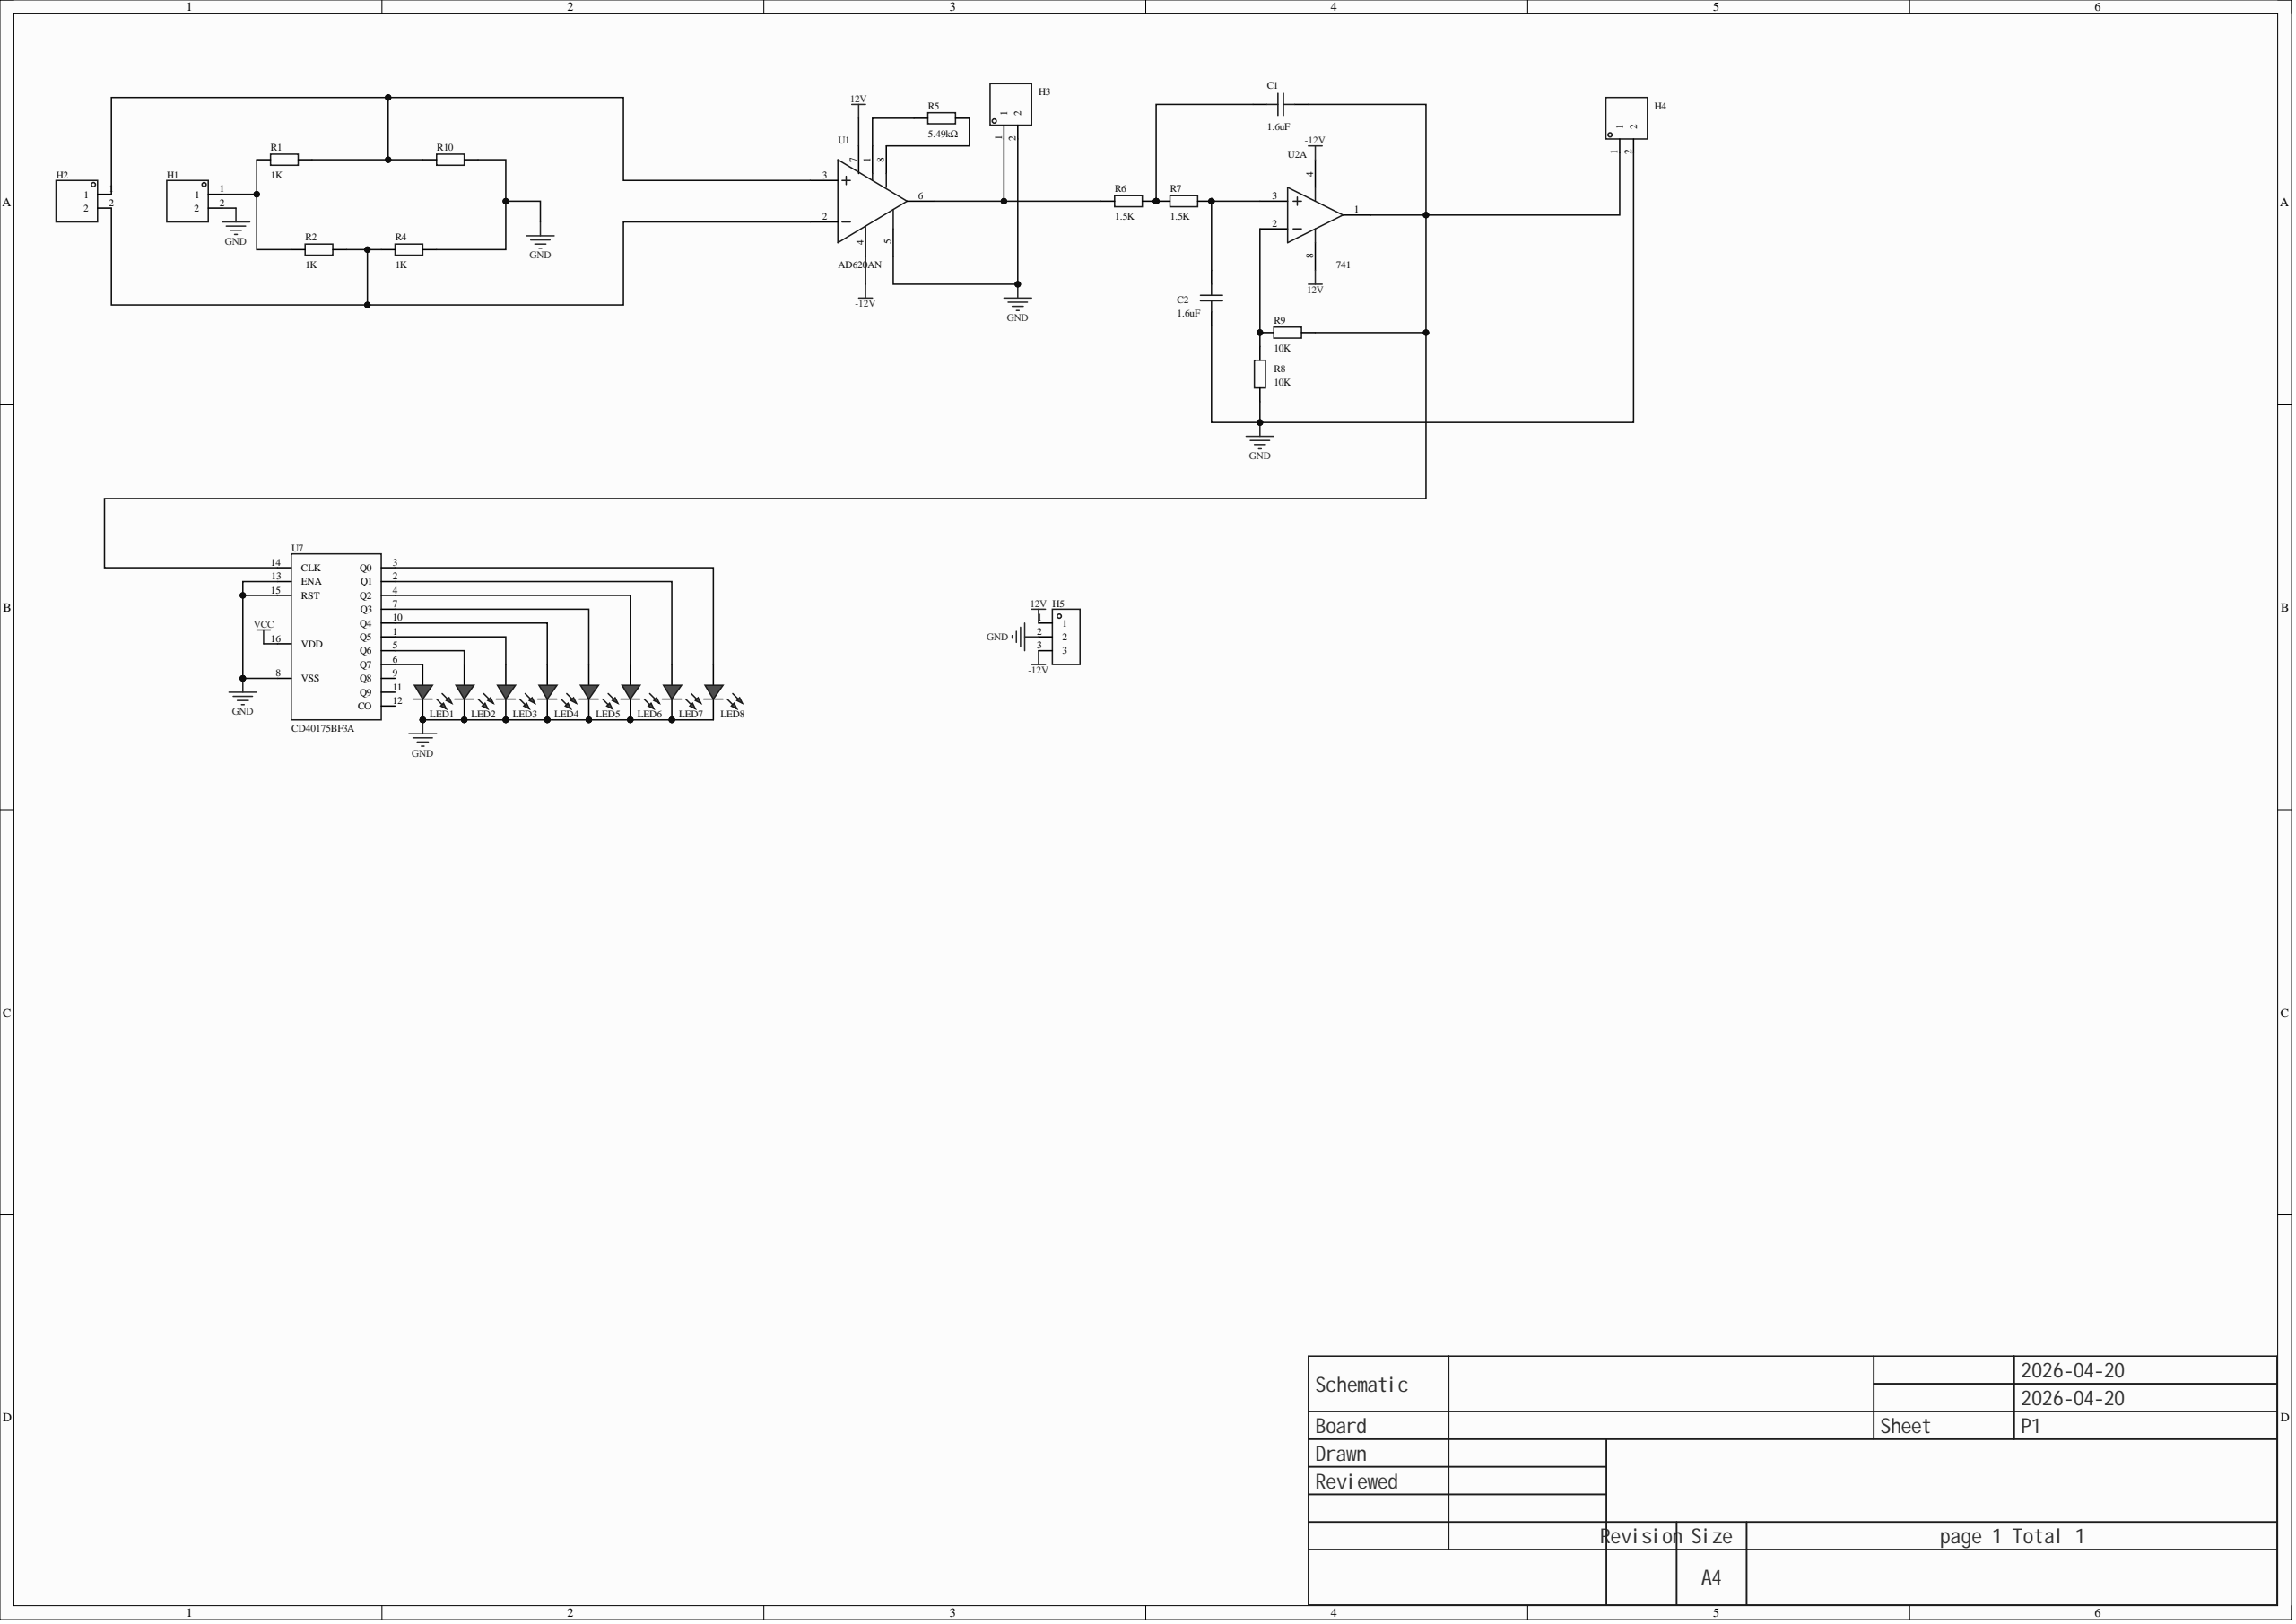Circuit board | Altium Designer | 27 parts | 21 nets
Bill of materials:
Comment,Description,Designator,Footprint,LibRef,Quantity
"1.6uF","","C1, C2","C0603","CAP_0603","2"
"","","H1, H2, H3, H4","HDR-TH_2P-P2.54-V-M-1","HDR-M_2.54_1x2P","4"
"","","H5","HDR-TH_3P-P2.54-V-F","HDR-F_2.54_1x3P","1"
"","","LED1, LED2, LED3, LED4, LED5, LED6, LED7, LED8","LED_TH-3mm","LED_TH-R_3mm","8"
"1K","","R1, R2, R4","R0603","Res_0603","3"
"5.49kΩ","","R5","R0603","Res_0603","1"
"1.5K","","R6, R7","R0603","Res_0603","2"
"10K","","R8, R9","R0603","Res_0603","2"
"10kΩ","","R10","Res_1/8W","Res_AXIAL-1/8W","1"
"AD620AN","Amplifier count: single; CMRR: 100dB; input bias current (Ib): 500pA; input offset voltage (Vos): 30uV; gain-bandwidth product (GBP): -; slew rate (SR): 0.75V/us; bandwidth (-3dB): 120kHz;","U1","DIP-8_L9.3-W6.4-P2.54-LS7.6-BL","AD620ANZ","1"
"741","Amplifier count: 2; rail-to-rail: -; gain-bandwidth product (GBW): 1MHz; input offset voltage (Vos): 2mV; slew rate (SR): -; input bias current (Ib): 50nA;","U2","PDIP-8_L10.2-W6.5-P2.54-LS7.6-BL","LM358AN/NOPB","1"
"CD40175BF3A","CD40175B-MIL CMOS quad D-type flip-flop","U7","CDIP-16_L21.4-W6.8-P2.54-LS7.8-BL","CD40175BF3A","1"
Netlist (Protel format):
[
C1
C0603
1.6uF



]
[
C2
C0603
1.6uF



]
[
H1
HDR-TH_2P-P2.54-V-M-1




]
[
H2
HDR-TH_2P-P2.54-V-M-1




]
[
H3
HDR-TH_2P-P2.54-V-M-1




]
[
H4
HDR-TH_2P-P2.54-V-M-1




]
[
H5
HDR-TH_3P-P2.54-V-F




]
[
LED1
LED_TH-3mm




]
[
LED2
LED_TH-3mm




]
[
LED3
LED_TH-3mm




]
[
LED4
LED_TH-3mm




]
[
LED5
LED_TH-3mm




]
[
LED6
LED_TH-3mm




]
[
LED7
LED_TH-3mm




]
[
LED8
LED_TH-3mm




]
[
R1
R0603
1K



]
[
R2
R0603
1K



]
[
R4
R0603
1K



]
[
R5
R0603
5.49kΩ



]
[
R6
R0603
1.5K



]
[
R7
R0603
1.5K



]
[
R8
R0603
10K



]
[
R9
R0603
10K



]
[
R10
Res_1/8W
10kΩ



]
[
U1
DIP-8_L9.3-W6.4-P2.54-LS7.6-BL
AD620AN



]
[
U2
PDIP-8_L10.2-W6.5-P2.54-LS7.6-BL
741



]
[
U7
CDIP-16_L21.4-W6.8-P2.54-LS7.8-BL
CD40175BF3A



]
(
NetR8_2
R8-2
R9-2
U2-2
)
(
NetR5_2
R5-2
U1-8
)
(
NetR5_1
R5-1
U1-1
)
(
NetLED8_1
LED8-1
U7-3
)
(
NetLED7_1
LED7-1
U7-2
)
(
NetLED6_1
LED6-1
U7-4
)
(
NetLED5_1
LED5-1
U7-7
)
(
NetLED4_1
LED4-1
U7-10
)
(
NetLED3_1
LED3-1
U7-1
)
(
NetLED2_1
LED2-1
U7-5
)
(
NetLED1_1
LED1-1
U7-6
)
(
NetH3_1
H3-1
R6-2
U1-6
)
(
NetH2_2
H2-2
R2-2
R4-1
U1-2
)
(
NetH2_1
H2-1
R1-2
R10-1
U1-3
)
(
NetH1_1
H1-1
R1-1
R2-1
)
(
NetC2_2
C2-2
R7-1
U2-3
)
(
NetC1_2
C1-2
H4-1
R9-1
U2-1
U7-14
)
(
NetC1_1
C1-1
R6-1
R7-2
)
(
GND
C2-1
H1-2
H3-2
H4-2
H5-2
LED1-2
LED2-2
LED3-2
LED4-2
LED5-2
LED6-2
LED7-2
LED8-2
R4-2
R8-1
R10-2
U1-5
U7-8
U7-13
U7-15
)
(
-12V
H5-3
U1-4
U2-4
)
(
12V
H5-1
U1-7
U2-8
)